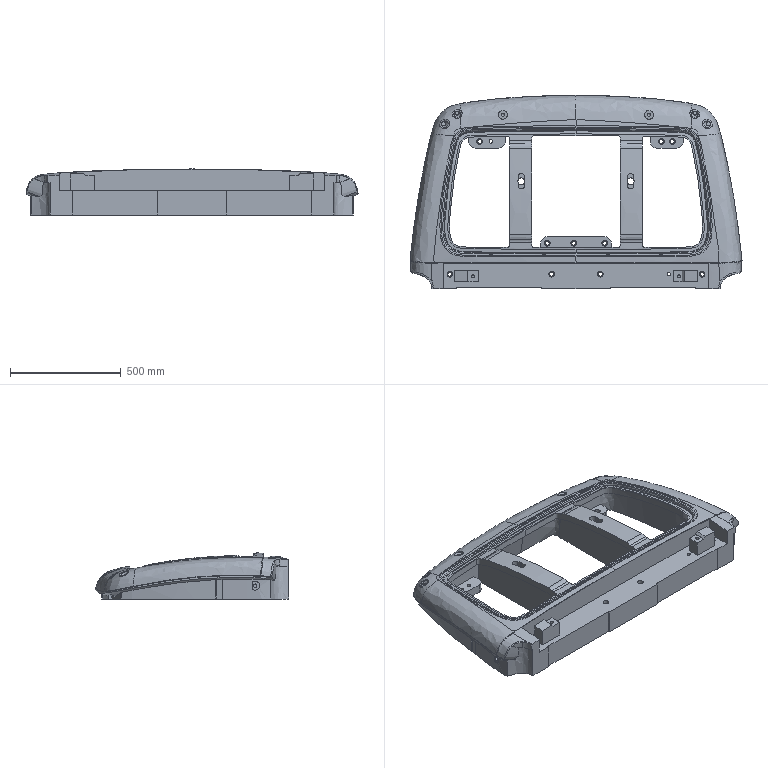Part | NX | features solid 2 | 1 solid | 491 faces | box 1500 x 873.218 x 208.055 mm | volume 92137603 mm3 | spline 259 | plane 136 | cylinder 84 | sphere 10 | cone 2 | commonest cylinder face diameters 6 x28 17.5 x10 26 x6 60 x6 6.004 x4 10 x4